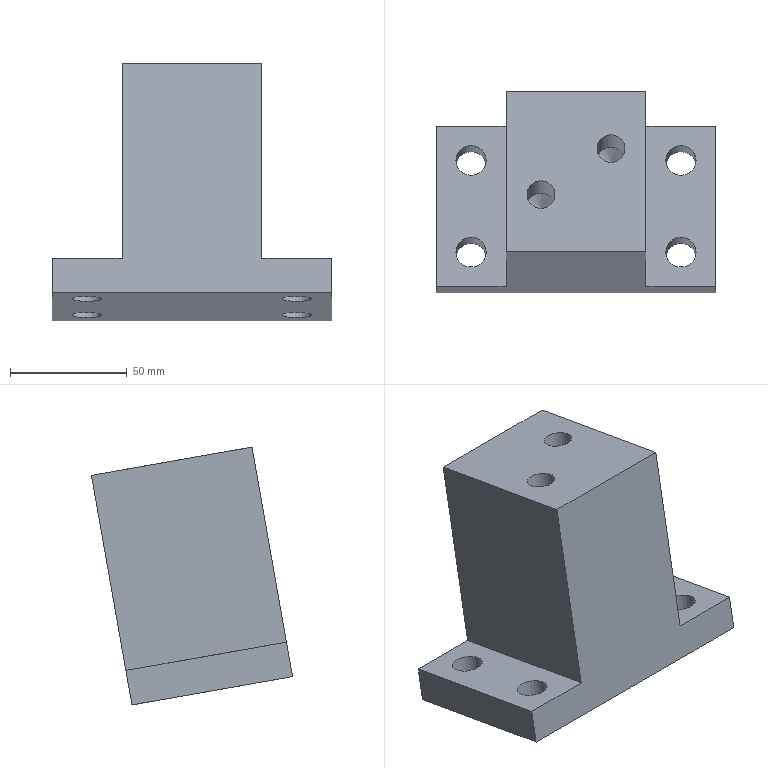Part | NX | features solid 2 | 1 solid | 18 faces | box 120 x 86.301 x 110.636 mm | volume 467978 mm3 | plane 10 | cylinder 6 | cone 2 | commonest cylinder face diameters 13 x4 12 x2
STEP:
#1=CARTESIAN_POINT('',(-73.5,-790.701,56.704));
#2=VERTEX_POINT('',#1);
#3=CARTESIAN_POINT('',(-73.5,-775.941,140.412));
#4=VERTEX_POINT('',#3);
#5=CARTESIAN_POINT('',(-73.5,-776.809,135.488));
#6=DIRECTION('',(0.,0.1736,0.9848));
#7=VECTOR('',#6,1000.);
#8=LINE('',#5,#7);
#9=EDGE_CURVE('',#2,#4,#8,.T.);
#10=ORIENTED_EDGE('',*,*,#9,.T.);
#11=CARTESIAN_POINT('',(-13.5,-775.941,140.412));
#12=VERTEX_POINT('',#11);
#13=CARTESIAN_POINT('',(-43.5,-775.941,140.412));
#14=DIRECTION('',(1.,0.,0.));
#15=VECTOR('',#14,1000.);
#16=LINE('',#13,#15);
#17=EDGE_CURVE('',#4,#12,#16,.T.);
#18=ORIENTED_EDGE('',*,*,#17,.T.);
#19=CARTESIAN_POINT('',(-13.5,-790.701,56.704));
#20=VERTEX_POINT('',#19);
#21=CARTESIAN_POINT('',(-13.5,-776.809,135.488));
#22=DIRECTION('',(0.,0.1736,0.9848));
#23=VECTOR('',#22,1000.);
#24=LINE('',#21,#23);
#25=EDGE_CURVE('',#20,#12,#24,.T.);
#26=ORIENTED_EDGE('',*,*,#25,.F.);
#27=CARTESIAN_POINT('',(16.5,-790.701,56.704));
#28=VERTEX_POINT('',#27);
#29=CARTESIAN_POINT('',(-43.5,-790.701,56.704));
#30=DIRECTION('',(-1.,0.,0.));
#31=VECTOR('',#30,1000.);
#32=LINE('',#29,#31);
#33=EDGE_CURVE('',#28,#20,#32,.T.);
#34=ORIENTED_EDGE('',*,*,#33,.F.);
#35=CARTESIAN_POINT('',(16.5,-793.306,41.932));
#36=VERTEX_POINT('',#35);
#37=CARTESIAN_POINT('',(16.5,-793.306,41.932));
#38=DIRECTION('',(0.,0.1736,0.9848));
#39=VECTOR('',#38,1000.);
#40=LINE('',#37,#39);
#41=EDGE_CURVE('',#36,#28,#40,.T.);
#42=ORIENTED_EDGE('',*,*,#41,.F.);
#43=CARTESIAN_POINT('',(-103.5,-793.306,41.932));
#44=VERTEX_POINT('',#43);
#45=CARTESIAN_POINT('',(-43.5,-793.306,41.932));
#46=DIRECTION('',(1.,0.,0.));
#47=VECTOR('',#46,1000.);
#48=LINE('',#45,#47);
#49=EDGE_CURVE('',#44,#36,#48,.T.);
#50=ORIENTED_EDGE('',*,*,#49,.F.);
#51=CARTESIAN_POINT('',(-103.5,-790.701,56.704));
#52=VERTEX_POINT('',#51);
#53=CARTESIAN_POINT('',(-103.5,-793.306,41.932));
#54=DIRECTION('',(0.,0.1736,0.9848));
#55=VECTOR('',#54,1000.);
#56=LINE('',#53,#55);
#57=EDGE_CURVE('',#44,#52,#56,.T.);
#58=ORIENTED_EDGE('',*,*,#57,.T.);
#59=CARTESIAN_POINT('',(-43.5,-790.701,56.704));
#60=DIRECTION('',(-1.,0.,0.));
#61=VECTOR('',#60,1000.);
#62=LINE('',#59,#61);
#63=EDGE_CURVE('',#2,#52,#62,.T.);
#64=ORIENTED_EDGE('',*,*,#63,.F.);
#65=EDGE_LOOP('',(#10,#18,#26,#34,#42,#50,#58,#64));
#66=FACE_BOUND('',#65,.T.);
#67=CARTESIAN_POINT('',(-43.5,-793.306,41.932));
#68=DIRECTION('',(0.,0.9848,-0.1736));
#69=DIRECTION('',(0.,-0.1736,-0.9848));
#70=AXIS2_PLACEMENT_3D('',#67,#68,#69);
#71=PLANE('',#70);
#72=ADVANCED_FACE('',(#66),#71,.T.);
#73=CARTESIAN_POINT('',(-13.5,-859.638,68.859));
#74=VERTEX_POINT('',#73);
#75=CARTESIAN_POINT('',(-13.5,-844.878,152.568));
#76=VERTEX_POINT('',#75);
#77=CARTESIAN_POINT('',(-13.5,-845.746,147.644));
#78=DIRECTION('',(0.,0.1736,0.9848));
#79=VECTOR('',#78,1000.);
#80=LINE('',#77,#79);
#81=EDGE_CURVE('',#74,#76,#80,.T.);
#82=ORIENTED_EDGE('',*,*,#81,.T.);
#83=CARTESIAN_POINT('',(-73.5,-844.878,152.568));
#84=VERTEX_POINT('',#83);
#85=CARTESIAN_POINT('',(-43.5,-844.878,152.568));
#86=DIRECTION('',(-1.,0.,0.));
#87=VECTOR('',#86,1000.);
#88=LINE('',#85,#87);
#89=EDGE_CURVE('',#76,#84,#88,.T.);
#90=ORIENTED_EDGE('',*,*,#89,.T.);
#91=CARTESIAN_POINT('',(-73.5,-859.638,68.859));
#92=VERTEX_POINT('',#91);
#93=CARTESIAN_POINT('',(-73.5,-845.746,147.644));
#94=DIRECTION('',(0.,0.1736,0.9848));
#95=VECTOR('',#94,1000.);
#96=LINE('',#93,#95);
#97=EDGE_CURVE('',#92,#84,#96,.T.);
#98=ORIENTED_EDGE('',*,*,#97,.F.);
#99=CARTESIAN_POINT('',(-103.5,-859.638,68.859));
#100=VERTEX_POINT('',#99);
#101=CARTESIAN_POINT('',(-43.5,-859.638,68.859));
#102=DIRECTION('',(1.,0.,0.));
#103=VECTOR('',#102,1000.);
#104=LINE('',#101,#103);
#105=EDGE_CURVE('',#100,#92,#104,.T.);
#106=ORIENTED_EDGE('',*,*,#105,.F.);
#107=CARTESIAN_POINT('',(-103.5,-862.242,54.087));
#108=VERTEX_POINT('',#107);
#109=CARTESIAN_POINT('',(-103.5,-862.242,54.087));
#110=DIRECTION('',(0.,0.1736,0.9848));
#111=VECTOR('',#110,1000.);
#112=LINE('',#109,#111);
#113=EDGE_CURVE('',#108,#100,#112,.T.);
#114=ORIENTED_EDGE('',*,*,#113,.F.);
#115=CARTESIAN_POINT('',(16.5,-862.242,54.087));
#116=VERTEX_POINT('',#115);
#117=CARTESIAN_POINT('',(-43.5,-862.242,54.087));
#118=DIRECTION('',(-1.,0.,0.));
#119=VECTOR('',#118,1000.);
#120=LINE('',#117,#119);
#121=EDGE_CURVE('',#116,#108,#120,.T.);
#122=ORIENTED_EDGE('',*,*,#121,.F.);
#123=CARTESIAN_POINT('',(16.5,-859.638,68.859));
#124=VERTEX_POINT('',#123);
#125=CARTESIAN_POINT('',(16.5,-862.242,54.087));
#126=DIRECTION('',(0.,0.1736,0.9848));
#127=VECTOR('',#126,1000.);
#128=LINE('',#125,#127);
#129=EDGE_CURVE('',#116,#124,#128,.T.);
#130=ORIENTED_EDGE('',*,*,#129,.T.);
#131=CARTESIAN_POINT('',(-43.5,-859.638,68.859));
#132=DIRECTION('',(1.,0.,0.));
#133=VECTOR('',#132,1000.);
#134=LINE('',#131,#133);
#135=EDGE_CURVE('',#74,#124,#134,.T.);
#136=ORIENTED_EDGE('',*,*,#135,.F.);
#137=EDGE_LOOP('',(#82,#90,#98,#106,#114,#122,#130,#136));
#138=FACE_BOUND('',#137,.T.);
#139=CARTESIAN_POINT('',(-43.5,-862.242,54.087));
#140=DIRECTION('',(0.,-0.9848,0.1736));
#141=DIRECTION('',(0.,0.1736,0.9848));
#142=AXIS2_PLACEMENT_3D('',#139,#140,#141);
#143=PLANE('',#142);
#144=ADVANCED_FACE('',(#138),#143,.T.);
#145=ORIENTED_EDGE('',*,*,#97,.T.);
#146=CARTESIAN_POINT('',(-73.5,-775.941,140.412));
#147=DIRECTION('',(0.,0.9848,-0.1736));
#148=VECTOR('',#147,1000.);
#149=LINE('',#146,#148);
#150=EDGE_CURVE('',#84,#4,#149,.T.);
#151=ORIENTED_EDGE('',*,*,#150,.T.);
#152=ORIENTED_EDGE('',*,*,#9,.F.);
#153=CARTESIAN_POINT('',(-73.5,-790.701,56.704));
#154=DIRECTION('',(0.,-0.9848,0.1736));
#155=VECTOR('',#154,1000.);
#156=LINE('',#153,#155);
#157=EDGE_CURVE('',#2,#92,#156,.T.);
#158=ORIENTED_EDGE('',*,*,#157,.T.);
#159=EDGE_LOOP('',(#145,#151,#152,#158));
#160=FACE_BOUND('',#159,.T.);
#161=CARTESIAN_POINT('',(-73.5,-790.701,56.704));
#162=DIRECTION('',(-1.,0.,0.));
#163=DIRECTION('',(0.,0.1736,0.9848));
#164=AXIS2_PLACEMENT_3D('',#161,#162,#163);
#165=PLANE('',#164);
#166=ADVANCED_FACE('',(#160),#165,.T.);
#167=ORIENTED_EDGE('',*,*,#25,.T.);
#168=CARTESIAN_POINT('',(-13.5,-844.878,152.568));
#169=DIRECTION('',(0.,-0.9848,0.1736));
#170=VECTOR('',#169,1000.);
#171=LINE('',#168,#170);
#172=EDGE_CURVE('',#12,#76,#171,.T.);
#173=ORIENTED_EDGE('',*,*,#172,.T.);
#174=ORIENTED_EDGE('',*,*,#81,.F.);
#175=CARTESIAN_POINT('',(-13.5,-790.701,56.704));
#176=DIRECTION('',(0.,-0.9848,0.1736));
#177=VECTOR('',#176,1000.);
#178=LINE('',#175,#177);
#179=EDGE_CURVE('',#20,#74,#178,.T.);
#180=ORIENTED_EDGE('',*,*,#179,.F.);
#181=EDGE_LOOP('',(#167,#173,#174,#180));
#182=FACE_BOUND('',#181,.T.);
#183=CARTESIAN_POINT('',(-13.5,-859.638,68.859));
#184=DIRECTION('',(1.,0.,0.));
#185=DIRECTION('',(0.,-0.1736,-0.9848));
#186=AXIS2_PLACEMENT_3D('',#183,#184,#185);
#187=PLANE('',#186);
#188=ADVANCED_FACE('',(#182),#187,.T.);
#189=CARTESIAN_POINT('',(-95.,-844.866,66.254));
#190=VERTEX_POINT('',#189);
#191=CARTESIAN_POINT('',(-88.5,-844.866,66.254));
#192=DIRECTION('',(0.,0.1736,0.9848));
#193=DIRECTION('',(-1.,0.,0.));
#194=AXIS2_PLACEMENT_3D('',#191,#192,#193);
#195=CIRCLE('',#194,6.5);
#196=EDGE_CURVE('',#190,#190,#195,.T.);
#197=ORIENTED_EDGE('',*,*,#196,.F.);
#198=EDGE_LOOP('',(#197));
#199=FACE_BOUND('',#198,.T.);
#200=CARTESIAN_POINT('',(-95.,-805.473,59.308));
#201=VERTEX_POINT('',#200);
#202=CARTESIAN_POINT('',(-88.5,-805.473,59.308));
#203=DIRECTION('',(0.,0.1736,0.9848));
#204=DIRECTION('',(-1.,0.,0.));
#205=AXIS2_PLACEMENT_3D('',#202,#203,#204);
#206=CIRCLE('',#205,6.5);
#207=EDGE_CURVE('',#201,#201,#206,.T.);
#208=ORIENTED_EDGE('',*,*,#207,.F.);
#209=EDGE_LOOP('',(#208));
#210=FACE_BOUND('',#209,.T.);
#211=ORIENTED_EDGE('',*,*,#63,.T.);
#212=CARTESIAN_POINT('',(-103.5,-825.169,62.781));
#213=DIRECTION('',(0.,-0.9848,0.1736));
#214=VECTOR('',#213,1000.);
#215=LINE('',#212,#214);
#216=EDGE_CURVE('',#52,#100,#215,.T.);
#217=ORIENTED_EDGE('',*,*,#216,.T.);
#218=ORIENTED_EDGE('',*,*,#105,.T.);
#219=ORIENTED_EDGE('',*,*,#157,.F.);
#220=EDGE_LOOP('',(#211,#217,#218,#219));
#221=FACE_BOUND('',#220,.T.);
#222=CARTESIAN_POINT('',(-43.5,-825.169,62.781));
#223=DIRECTION('',(0.,0.1736,0.9848));
#224=DIRECTION('',(1.,0.,0.));
#225=AXIS2_PLACEMENT_3D('',#222,#223,#224);
#226=PLANE('',#225);
#227=ADVANCED_FACE('',(#199,#210,#221),#226,.T.);
#228=CARTESIAN_POINT('',(-5.,-844.866,66.254));
#229=VERTEX_POINT('',#228);
#230=CARTESIAN_POINT('',(1.5,-844.866,66.254));
#231=DIRECTION('',(0.,0.1736,0.9848));
#232=DIRECTION('',(-1.,0.,0.));
#233=AXIS2_PLACEMENT_3D('',#230,#231,#232);
#234=CIRCLE('',#233,6.5);
#235=EDGE_CURVE('',#229,#229,#234,.T.);
#236=ORIENTED_EDGE('',*,*,#235,.F.);
#237=EDGE_LOOP('',(#236));
#238=FACE_BOUND('',#237,.T.);
#239=CARTESIAN_POINT('',(-5.,-805.473,59.308));
#240=VERTEX_POINT('',#239);
#241=CARTESIAN_POINT('',(1.5,-805.473,59.308));
#242=DIRECTION('',(0.,0.1736,0.9848));
#243=DIRECTION('',(-1.,0.,0.));
#244=AXIS2_PLACEMENT_3D('',#241,#242,#243);
#245=CIRCLE('',#244,6.5);
#246=EDGE_CURVE('',#240,#240,#245,.T.);
#247=ORIENTED_EDGE('',*,*,#246,.F.);
#248=EDGE_LOOP('',(#247));
#249=FACE_BOUND('',#248,.T.);
#250=ORIENTED_EDGE('',*,*,#179,.T.);
#251=ORIENTED_EDGE('',*,*,#135,.T.);
#252=CARTESIAN_POINT('',(16.5,-825.169,62.781));
#253=DIRECTION('',(0.,0.9848,-0.1736));
#254=VECTOR('',#253,1000.);
#255=LINE('',#252,#254);
#256=EDGE_CURVE('',#124,#28,#255,.T.);
#257=ORIENTED_EDGE('',*,*,#256,.T.);
#258=ORIENTED_EDGE('',*,*,#33,.T.);
#259=EDGE_LOOP('',(#250,#251,#257,#258));
#260=FACE_BOUND('',#259,.T.);
#261=CARTESIAN_POINT('',(-43.5,-825.169,62.781));
#262=DIRECTION('',(0.,0.1736,0.9848));
#263=DIRECTION('',(1.,0.,0.));
#264=AXIS2_PLACEMENT_3D('',#261,#262,#263);
#265=PLANE('',#264);
#266=ADVANCED_FACE('',(#238,#249,#260),#265,.T.);
#267=ORIENTED_EDGE('',*,*,#57,.F.);
#268=CARTESIAN_POINT('',(-103.5,-827.774,48.009));
#269=DIRECTION('',(0.,0.9848,-0.1736));
#270=VECTOR('',#269,1000.);
#271=LINE('',#268,#270);
#272=EDGE_CURVE('',#108,#44,#271,.T.);
#273=ORIENTED_EDGE('',*,*,#272,.F.);
#274=ORIENTED_EDGE('',*,*,#113,.T.);
#275=ORIENTED_EDGE('',*,*,#216,.F.);
#276=EDGE_LOOP('',(#267,#273,#274,#275));
#277=FACE_BOUND('',#276,.T.);
#278=CARTESIAN_POINT('',(-103.5,-827.774,48.009));
#279=DIRECTION('',(-1.,0.,0.));
#280=DIRECTION('',(0.,0.1736,0.9848));
#281=AXIS2_PLACEMENT_3D('',#278,#279,#280);
#282=PLANE('',#281);
#283=ADVANCED_FACE('',(#277),#282,.T.);
#284=CARTESIAN_POINT('',(-5.,-847.47,51.482));
#285=VERTEX_POINT('',#284);
#286=CARTESIAN_POINT('',(1.5,-847.47,51.482));
#287=DIRECTION('',(0.,0.1736,0.9848));
#288=DIRECTION('',(-1.,0.,0.));
#289=AXIS2_PLACEMENT_3D('',#286,#287,#288);
#290=CIRCLE('',#289,6.5);
#291=EDGE_CURVE('',#285,#285,#290,.T.);
#292=ORIENTED_EDGE('',*,*,#291,.T.);
#293=EDGE_LOOP('',(#292));
#294=FACE_BOUND('',#293,.T.);
#295=CARTESIAN_POINT('',(-5.,-808.078,44.536));
#296=VERTEX_POINT('',#295);
#297=CARTESIAN_POINT('',(1.5,-808.078,44.536));
#298=DIRECTION('',(0.,0.1736,0.9848));
#299=DIRECTION('',(-1.,0.,0.));
#300=AXIS2_PLACEMENT_3D('',#297,#298,#299);
#301=CIRCLE('',#300,6.5);
#302=EDGE_CURVE('',#296,#296,#301,.T.);
#303=ORIENTED_EDGE('',*,*,#302,.T.);
#304=EDGE_LOOP('',(#303));
#305=FACE_BOUND('',#304,.T.);
#306=CARTESIAN_POINT('',(-95.,-847.47,51.482));
#307=VERTEX_POINT('',#306);
#308=CARTESIAN_POINT('',(-88.5,-847.47,51.482));
#309=DIRECTION('',(0.,0.1736,0.9848));
#310=DIRECTION('',(-1.,0.,0.));
#311=AXIS2_PLACEMENT_3D('',#308,#309,#310);
#312=CIRCLE('',#311,6.5);
#313=EDGE_CURVE('',#307,#307,#312,.T.);
#314=ORIENTED_EDGE('',*,*,#313,.T.);
#315=EDGE_LOOP('',(#314));
#316=FACE_BOUND('',#315,.T.);
#317=CARTESIAN_POINT('',(-95.,-808.078,44.536));
#318=VERTEX_POINT('',#317);
#319=CARTESIAN_POINT('',(-88.5,-808.078,44.536));
#320=DIRECTION('',(0.,0.1736,0.9848));
#321=DIRECTION('',(-1.,0.,0.));
#322=AXIS2_PLACEMENT_3D('',#319,#320,#321);
#323=CIRCLE('',#322,6.5);
#324=EDGE_CURVE('',#318,#318,#323,.T.);
#325=ORIENTED_EDGE('',*,*,#324,.T.);
#326=EDGE_LOOP('',(#325));
#327=FACE_BOUND('',#326,.T.);
#328=CARTESIAN_POINT('',(16.5,-827.774,48.009));
#329=DIRECTION('',(0.,-0.9848,0.1736));
#330=VECTOR('',#329,1000.);
#331=LINE('',#328,#330);
#332=EDGE_CURVE('',#36,#116,#331,.T.);
#333=ORIENTED_EDGE('',*,*,#332,.T.);
#334=ORIENTED_EDGE('',*,*,#121,.T.);
#335=ORIENTED_EDGE('',*,*,#272,.T.);
#336=ORIENTED_EDGE('',*,*,#49,.T.);
#337=EDGE_LOOP('',(#333,#334,#335,#336));
#338=FACE_BOUND('',#337,.T.);
#339=CARTESIAN_POINT('',(-43.5,-827.774,48.009));
#340=DIRECTION('',(0.,-0.1736,-0.9848));
#341=DIRECTION('',(-1.,0.,0.));
#342=AXIS2_PLACEMENT_3D('',#339,#340,#341);
#343=PLANE('',#342);
#344=ADVANCED_FACE('',(#294,#305,#316,#327,#338),#343,.T.);
#345=ORIENTED_EDGE('',*,*,#332,.F.);
#346=ORIENTED_EDGE('',*,*,#41,.T.);
#347=ORIENTED_EDGE('',*,*,#256,.F.);
#348=ORIENTED_EDGE('',*,*,#129,.F.);
#349=EDGE_LOOP('',(#345,#346,#347,#348));
#350=FACE_BOUND('',#349,.T.);
#351=CARTESIAN_POINT('',(16.5,-827.774,48.009));
#352=DIRECTION('',(1.,0.,0.));
#353=DIRECTION('',(0.,-0.1736,-0.9848));
#354=AXIS2_PLACEMENT_3D('',#351,#352,#353);
#355=PLANE('',#354);
#356=ADVANCED_FACE('',(#350),#355,.T.);
#357=ORIENTED_EDGE('',*,*,#324,.F.);
#358=EDGE_LOOP('',(#357));
#359=FACE_BOUND('',#358,.T.);
#360=ORIENTED_EDGE('',*,*,#207,.T.);
#361=EDGE_LOOP('',(#360));
#362=FACE_BOUND('',#361,.T.);
#363=CARTESIAN_POINT('',(-88.5,-805.473,59.308));
#364=DIRECTION('',(0.,-0.1736,-0.9848));
#365=DIRECTION('',(-1.,0.,0.));
#366=AXIS2_PLACEMENT_3D('',#363,#364,#365);
#367=CYLINDRICAL_SURFACE('',#366,6.5);
#368=ADVANCED_FACE('',(#359,#362),#367,.F.);
#369=ORIENTED_EDGE('',*,*,#313,.F.);
#370=EDGE_LOOP('',(#369));
#371=FACE_BOUND('',#370,.T.);
#372=ORIENTED_EDGE('',*,*,#196,.T.);
#373=EDGE_LOOP('',(#372));
#374=FACE_BOUND('',#373,.T.);
#375=CARTESIAN_POINT('',(-88.5,-844.866,66.254));
#376=DIRECTION('',(0.,-0.1736,-0.9848));
#377=DIRECTION('',(-1.,0.,0.));
#378=AXIS2_PLACEMENT_3D('',#375,#376,#377);
#379=CYLINDRICAL_SURFACE('',#378,6.5);
#380=ADVANCED_FACE('',(#371,#374),#379,.F.);
#381=ORIENTED_EDGE('',*,*,#302,.F.);
#382=EDGE_LOOP('',(#381));
#383=FACE_BOUND('',#382,.T.);
#384=ORIENTED_EDGE('',*,*,#246,.T.);
#385=EDGE_LOOP('',(#384));
#386=FACE_BOUND('',#385,.T.);
#387=CARTESIAN_POINT('',(1.5,-805.473,59.308));
#388=DIRECTION('',(0.,-0.1736,-0.9848));
#389=DIRECTION('',(-1.,0.,0.));
#390=AXIS2_PLACEMENT_3D('',#387,#388,#389);
#391=CYLINDRICAL_SURFACE('',#390,6.5);
#392=ADVANCED_FACE('',(#383,#386),#391,.F.);
#393=ORIENTED_EDGE('',*,*,#291,.F.);
#394=EDGE_LOOP('',(#393));
#395=FACE_BOUND('',#394,.T.);
#396=ORIENTED_EDGE('',*,*,#235,.T.);
#397=EDGE_LOOP('',(#396));
#398=FACE_BOUND('',#397,.T.);
#399=CARTESIAN_POINT('',(1.5,-844.866,66.254));
#400=DIRECTION('',(0.,-0.1736,-0.9848));
#401=DIRECTION('',(-1.,0.,0.));
#402=AXIS2_PLACEMENT_3D('',#399,#400,#401);
#403=CYLINDRICAL_SURFACE('',#402,6.5);
#404=ADVANCED_FACE('',(#395,#398),#403,.F.);
#405=CARTESIAN_POINT('',(-28.5,-806.47,145.795));
#406=VERTEX_POINT('',#405);
#407=CARTESIAN_POINT('',(-28.5,-800.561,144.754));
#408=DIRECTION('',(0.,0.1736,0.9848));
#409=DIRECTION('',(0.,-0.9848,0.1736));
#410=AXIS2_PLACEMENT_3D('',#407,#408,#409);
#411=CIRCLE('',#410,6.);
#412=EDGE_CURVE('',#406,#406,#411,.T.);
#413=ORIENTED_EDGE('',*,*,#412,.F.);
#414=EDGE_LOOP('',(#413));
#415=FACE_BOUND('',#414,.T.);
#416=CARTESIAN_POINT('',(-58.5,-826.166,149.268));
#417=VERTEX_POINT('',#416);
#418=CARTESIAN_POINT('',(-58.5,-820.257,148.227));
#419=DIRECTION('',(0.,0.1736,0.9848));
#420=DIRECTION('',(0.,-0.9848,0.1736));
#421=AXIS2_PLACEMENT_3D('',#418,#419,#420);
#422=CIRCLE('',#421,6.);
#423=EDGE_CURVE('',#417,#417,#422,.T.);
#424=ORIENTED_EDGE('',*,*,#423,.F.);
#425=EDGE_LOOP('',(#424));
#426=FACE_BOUND('',#425,.T.);
#427=ORIENTED_EDGE('',*,*,#150,.F.);
#428=ORIENTED_EDGE('',*,*,#89,.F.);
#429=ORIENTED_EDGE('',*,*,#172,.F.);
#430=ORIENTED_EDGE('',*,*,#17,.F.);
#431=EDGE_LOOP('',(#427,#428,#429,#430));
#432=FACE_BOUND('',#431,.T.);
#433=CARTESIAN_POINT('',(-73.5,-736.549,133.466));
#434=DIRECTION('',(0.,0.1736,0.9848));
#435=DIRECTION('',(0.,0.9848,-0.1736));
#436=AXIS2_PLACEMENT_3D('',#433,#434,#435);
#437=PLANE('',#436);
#438=ADVANCED_FACE('',(#415,#426,#432),#437,.T.);
#439=CARTESIAN_POINT('',(-58.5,-831.376,119.724));
#440=VERTEX_POINT('',#439);
#441=CARTESIAN_POINT('',(-58.5,-825.467,118.682));
#442=DIRECTION('',(0.,0.1736,0.9848));
#443=DIRECTION('',(0.,-0.9848,0.1736));
#444=AXIS2_PLACEMENT_3D('',#441,#442,#443);
#445=CIRCLE('',#444,6.);
#446=EDGE_CURVE('',#440,#440,#445,.T.);
#447=ORIENTED_EDGE('',*,*,#446,.T.);
#448=EDGE_LOOP('',(#447));
#449=FACE_BOUND('',#448,.T.);
#450=CARTESIAN_POINT('',(-58.5,-826.093,115.132));
#451=VERTEX_POINT('',#450);
#452=VERTEX_LOOP('',#451);
#453=FACE_BOUND('',#452,.T.);
#454=CARTESIAN_POINT('',(-58.5,-825.467,118.682));
#455=DIRECTION('',(0.,0.1736,0.9848));
#456=DIRECTION('',(0.,0.9848,-0.1736));
#457=AXIS2_PLACEMENT_3D('',#454,#455,#456);
#458=CONICAL_SURFACE('',#457,6.,1.03);
#459=ADVANCED_FACE('',(#449,#453),#458,.F.);
#460=ORIENTED_EDGE('',*,*,#446,.F.);
#461=EDGE_LOOP('',(#460));
#462=FACE_BOUND('',#461,.T.);
#463=ORIENTED_EDGE('',*,*,#423,.T.);
#464=EDGE_LOOP('',(#463));
#465=FACE_BOUND('',#464,.T.);
#466=CARTESIAN_POINT('',(-58.5,-820.257,148.227));
#467=DIRECTION('',(0.,-0.1736,-0.9848));
#468=DIRECTION('',(0.,-0.9848,0.1736));
#469=AXIS2_PLACEMENT_3D('',#466,#467,#468);
#470=CYLINDRICAL_SURFACE('',#469,6.);
#471=ADVANCED_FACE('',(#462,#465),#470,.F.);
#472=CARTESIAN_POINT('',(-28.5,-811.679,116.251));
#473=VERTEX_POINT('',#472);
#474=CARTESIAN_POINT('',(-28.5,-805.771,115.209));
#475=DIRECTION('',(0.,0.1736,0.9848));
#476=DIRECTION('',(0.,-0.9848,0.1736));
#477=AXIS2_PLACEMENT_3D('',#474,#475,#476);
#478=CIRCLE('',#477,6.);
#479=EDGE_CURVE('',#473,#473,#478,.T.);
#480=ORIENTED_EDGE('',*,*,#479,.T.);
#481=EDGE_LOOP('',(#480));
#482=FACE_BOUND('',#481,.T.);
#483=CARTESIAN_POINT('',(-28.5,-806.397,111.659));
#484=VERTEX_POINT('',#483);
#485=VERTEX_LOOP('',#484);
#486=FACE_BOUND('',#485,.T.);
#487=CARTESIAN_POINT('',(-28.5,-805.771,115.209));
#488=DIRECTION('',(0.,0.1736,0.9848));
#489=DIRECTION('',(0.,0.9848,-0.1736));
#490=AXIS2_PLACEMENT_3D('',#487,#488,#489);
#491=CONICAL_SURFACE('',#490,6.,1.03);
#492=ADVANCED_FACE('',(#482,#486),#491,.F.);
#493=ORIENTED_EDGE('',*,*,#479,.F.);
#494=EDGE_LOOP('',(#493));
#495=FACE_BOUND('',#494,.T.);
#496=ORIENTED_EDGE('',*,*,#412,.T.);
#497=EDGE_LOOP('',(#496));
#498=FACE_BOUND('',#497,.T.);
#499=CARTESIAN_POINT('',(-28.5,-800.561,144.754));
#500=DIRECTION('',(0.,-0.1736,-0.9848));
#501=DIRECTION('',(0.,-0.9848,0.1736));
#502=AXIS2_PLACEMENT_3D('',#499,#500,#501);
#503=CYLINDRICAL_SURFACE('',#502,6.);
#504=ADVANCED_FACE('',(#495,#498),#503,.F.);
#505=CLOSED_SHELL('',(#72,#144,#166,#188,#227,#266,#283,#344,#356,#368,#380,#392,#404,#438,#459,#471,#492,#504));
#506=MANIFOLD_SOLID_BREP('',#505);
#507=(LENGTH_UNIT()NAMED_UNIT(*)SI_UNIT(.MILLI.,.METRE.));
#508=UNCERTAINTY_MEASURE_WITH_UNIT(LENGTH_MEASURE(0.00001),#507,'','');
#509=(NAMED_UNIT(*)PLANE_ANGLE_UNIT()SI_UNIT($,.RADIAN.));
#510=(NAMED_UNIT(*)SI_UNIT($,.STERADIAN.)SOLID_ANGLE_UNIT());
#511=(GEOMETRIC_REPRESENTATION_CONTEXT(3)GLOBAL_UNCERTAINTY_ASSIGNED_CONTEXT((#508))GLOBAL_UNIT_ASSIGNED_CONTEXT((#507,#509,#510))REPRESENTATION_CONTEXT('',''));
#512=ADVANCED_BREP_SHAPE_REPRESENTATION('',(#506),#511);